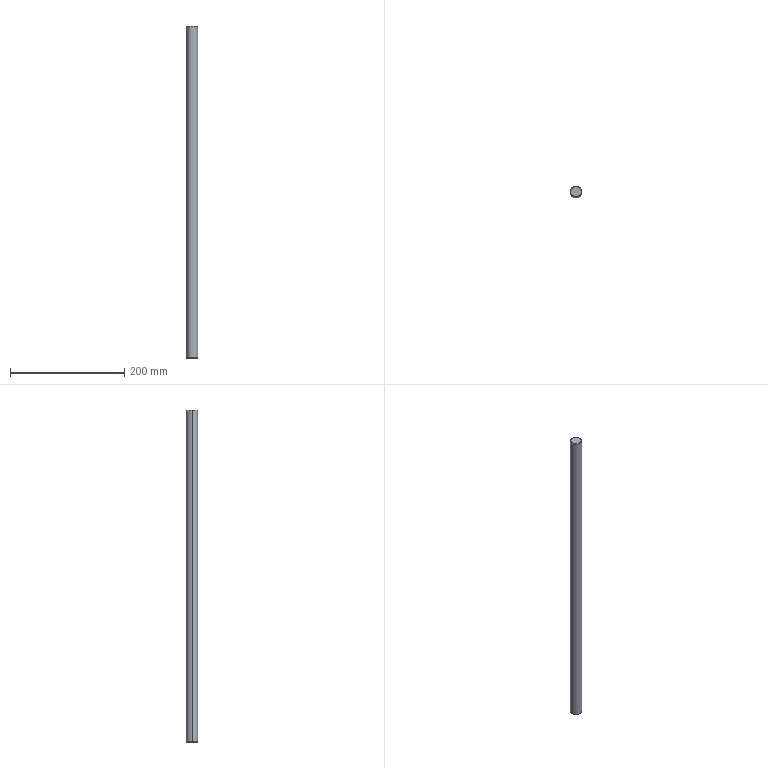Part | STEP file | 20309 | 1 solid | 8 faces | box 20 x 20 x 580 mm | volume 182152 mm3 | cone 4 | plane 2 | cylinder 2 | commonest cylinder face diameters 20 x2
STEP:
#1=CARTESIAN_POINT('',(9.,0.,580.));
#2=VERTEX_POINT('',#1);
#3=CARTESIAN_POINT('',(-9.,0.000000111,580.));
#4=VERTEX_POINT('',#3);
#5=CARTESIAN_POINT('',(0.,0.,580.));
#6=DIRECTION('',(0.,0.,1.));
#7=AXIS2_PLACEMENT_3D('',#5,#6,$);
#8=CIRCLE('',#7,9.);
#9=EDGE_CURVE('',#2,#4,#8,.T.);
#10=ORIENTED_EDGE('',*,*,#9,.T.);
#11=CARTESIAN_POINT('',(0.,0.,580.));
#12=DIRECTION('',(0.,0.,1.));
#13=AXIS2_PLACEMENT_3D('',#11,#12,$);
#14=CIRCLE('',#13,9.);
#15=EDGE_CURVE('',#4,#2,#14,.T.);
#16=ORIENTED_EDGE('',*,*,#15,.T.);
#17=EDGE_LOOP('',(#10,#16));
#18=FACE_OUTER_BOUND('',#17,.T.);
#19=CARTESIAN_POINT('',(0.,0.,580.));
#20=DIRECTION('',(0.,0.,1.));
#21=DIRECTION('',(1.,0.,0.));
#22=AXIS2_PLACEMENT_3D('',#19,#20,#21);
#23=PLANE('',#22);
#24=ADVANCED_FACE('',(#18),#23,.T.);
#25=CARTESIAN_POINT('',(10.,0.,579.));
#26=VERTEX_POINT('',#25);
#27=CARTESIAN_POINT('',(9.5,0.,579.5));
#28=DIRECTION('',(0.7071,0.,-0.7071));
#29=VECTOR('',#28,1.);
#30=LINE('',#27,#29);
#31=EDGE_CURVE('',#2,#26,#30,.T.);
#32=ORIENTED_EDGE('',*,*,#31,.T.);
#33=CARTESIAN_POINT('',(-10.,0.,579.));
#34=VERTEX_POINT('',#33);
#35=CARTESIAN_POINT('',(0.,0.,579.));
#36=DIRECTION('',(0.,0.,1.));
#37=AXIS2_PLACEMENT_3D('',#35,#36,$);
#38=CIRCLE('',#37,10.);
#39=EDGE_CURVE('',#26,#34,#38,.T.);
#40=ORIENTED_EDGE('',*,*,#39,.T.);
#41=CARTESIAN_POINT('',(-9.5,0.,579.5));
#42=DIRECTION('',(-0.7071,0.,-0.7071));
#43=VECTOR('',#42,1.);
#44=LINE('',#41,#43);
#45=EDGE_CURVE('',#4,#34,#44,.T.);
#46=ORIENTED_EDGE('',*,*,#45,.F.);
#47=ORIENTED_EDGE('',*,*,#9,.F.);
#48=EDGE_LOOP('',(#32,#40,#46,#47));
#49=FACE_OUTER_BOUND('',#48,.T.);
#50=CARTESIAN_POINT('',(0.,0.,589.));
#51=DIRECTION('',(0.,0.,-1.));
#52=DIRECTION('',(1.,0.,0.));
#53=AXIS2_PLACEMENT_3D('',#50,#51,#52);
#54=CONICAL_SURFACE('',#53,0.,0.7854);
#55=ADVANCED_FACE('',(#49),#54,.T.);
#56=ORIENTED_EDGE('',*,*,#45,.T.);
#57=CARTESIAN_POINT('',(0.,0.,579.));
#58=DIRECTION('',(0.,0.,1.));
#59=AXIS2_PLACEMENT_3D('',#57,#58,$);
#60=CIRCLE('',#59,10.);
#61=EDGE_CURVE('',#34,#26,#60,.T.);
#62=ORIENTED_EDGE('',*,*,#61,.T.);
#63=ORIENTED_EDGE('',*,*,#31,.F.);
#64=ORIENTED_EDGE('',*,*,#15,.F.);
#65=EDGE_LOOP('',(#56,#62,#63,#64));
#66=FACE_OUTER_BOUND('',#65,.T.);
#67=CARTESIAN_POINT('',(0.,0.,589.));
#68=DIRECTION('',(0.,0.,-1.));
#69=DIRECTION('',(-0.9881,0.1539,0.));
#70=AXIS2_PLACEMENT_3D('',#67,#68,#69);
#71=CONICAL_SURFACE('',#70,0.,0.7854);
#72=ADVANCED_FACE('',(#66),#71,.T.);
#73=CARTESIAN_POINT('',(-9.,0.000000111,0.));
#74=VERTEX_POINT('',#73);
#75=CARTESIAN_POINT('',(9.,0.,0.));
#76=VERTEX_POINT('',#75);
#77=CARTESIAN_POINT('',(0.,0.,0.));
#78=DIRECTION('',(0.,0.,1.));
#79=AXIS2_PLACEMENT_3D('',#77,#78,$);
#80=CIRCLE('',#79,9.);
#81=EDGE_CURVE('',#74,#76,#80,.T.);
#82=ORIENTED_EDGE('',*,*,#81,.F.);
#83=CARTESIAN_POINT('',(0.,0.,0.));
#84=DIRECTION('',(0.,0.,1.));
#85=AXIS2_PLACEMENT_3D('',#83,#84,$);
#86=CIRCLE('',#85,9.);
#87=EDGE_CURVE('',#76,#74,#86,.T.);
#88=ORIENTED_EDGE('',*,*,#87,.F.);
#89=EDGE_LOOP('',(#82,#88));
#90=FACE_OUTER_BOUND('',#89,.T.);
#91=CARTESIAN_POINT('',(0.,0.,0.));
#92=DIRECTION('',(0.,0.,1.));
#93=DIRECTION('',(1.,0.,0.));
#94=AXIS2_PLACEMENT_3D('',#91,#92,#93);
#95=PLANE('',#94);
#96=ADVANCED_FACE('',(#90),#95,.F.);
#97=CARTESIAN_POINT('',(-10.,0.,1.));
#98=VERTEX_POINT('',#97);
#99=CARTESIAN_POINT('',(-10.,0.,290.));
#100=DIRECTION('',(0.,0.,1.));
#101=VECTOR('',#100,1.);
#102=LINE('',#99,#101);
#103=EDGE_CURVE('',#98,#34,#102,.T.);
#104=ORIENTED_EDGE('',*,*,#103,.T.);
#105=ORIENTED_EDGE('',*,*,#39,.F.);
#106=CARTESIAN_POINT('',(10.,0.,1.));
#107=VERTEX_POINT('',#106);
#108=CARTESIAN_POINT('',(10.,0.,290.));
#109=DIRECTION('',(0.,0.,1.));
#110=VECTOR('',#109,1.);
#111=LINE('',#108,#110);
#112=EDGE_CURVE('',#107,#26,#111,.T.);
#113=ORIENTED_EDGE('',*,*,#112,.F.);
#114=CARTESIAN_POINT('',(0.,0.,1.));
#115=DIRECTION('',(0.,0.,1.));
#116=AXIS2_PLACEMENT_3D('',#114,#115,$);
#117=CIRCLE('',#116,10.);
#118=EDGE_CURVE('',#107,#98,#117,.T.);
#119=ORIENTED_EDGE('',*,*,#118,.T.);
#120=EDGE_LOOP('',(#104,#105,#113,#119));
#121=FACE_OUTER_BOUND('',#120,.T.);
#122=CARTESIAN_POINT('',(0.,0.,290.));
#123=DIRECTION('',(0.,0.,1.));
#124=DIRECTION('',(1.,0.,0.));
#125=AXIS2_PLACEMENT_3D('',#122,#123,#124);
#126=CYLINDRICAL_SURFACE('',#125,10.);
#127=ADVANCED_FACE('',(#121),#126,.T.);
#128=ORIENTED_EDGE('',*,*,#112,.T.);
#129=ORIENTED_EDGE('',*,*,#61,.F.);
#130=ORIENTED_EDGE('',*,*,#103,.F.);
#131=CARTESIAN_POINT('',(0.,0.,1.));
#132=DIRECTION('',(0.,0.,1.));
#133=AXIS2_PLACEMENT_3D('',#131,#132,$);
#134=CIRCLE('',#133,10.);
#135=EDGE_CURVE('',#98,#107,#134,.T.);
#136=ORIENTED_EDGE('',*,*,#135,.T.);
#137=EDGE_LOOP('',(#128,#129,#130,#136));
#138=FACE_OUTER_BOUND('',#137,.T.);
#139=ADVANCED_FACE('',(#138),#126,.T.);
#140=CARTESIAN_POINT('',(9.5,0.,0.5));
#141=DIRECTION('',(0.7071,0.,0.7071));
#142=VECTOR('',#141,1.);
#143=LINE('',#140,#142);
#144=EDGE_CURVE('',#107,#76,#143,.F.);
#145=ORIENTED_EDGE('',*,*,#144,.T.);
#146=ORIENTED_EDGE('',*,*,#87,.T.);
#147=CARTESIAN_POINT('',(-9.5,0.000000117,0.5));
#148=DIRECTION('',(-0.7071,0.000000009,0.7071));
#149=VECTOR('',#148,1.);
#150=LINE('',#147,#149);
#151=EDGE_CURVE('',#98,#74,#150,.F.);
#152=ORIENTED_EDGE('',*,*,#151,.F.);
#153=ORIENTED_EDGE('',*,*,#118,.F.);
#154=EDGE_LOOP('',(#145,#146,#152,#153));
#155=FACE_OUTER_BOUND('',#154,.T.);
#156=CARTESIAN_POINT('',(0.,0.,-9.));
#157=DIRECTION('',(0.,0.,1.));
#158=DIRECTION('',(1.,0.,0.));
#159=AXIS2_PLACEMENT_3D('',#156,#157,#158);
#160=CONICAL_SURFACE('',#159,0.,0.7854);
#161=ADVANCED_FACE('',(#155),#160,.T.);
#162=ORIENTED_EDGE('',*,*,#151,.T.);
#163=ORIENTED_EDGE('',*,*,#81,.T.);
#164=ORIENTED_EDGE('',*,*,#144,.F.);
#165=ORIENTED_EDGE('',*,*,#135,.F.);
#166=EDGE_LOOP('',(#162,#163,#164,#165));
#167=FACE_OUTER_BOUND('',#166,.T.);
#168=CARTESIAN_POINT('',(0.,0.,-9.));
#169=DIRECTION('',(0.,0.,1.));
#170=DIRECTION('',(-0.9881,0.1539,0.));
#171=AXIS2_PLACEMENT_3D('',#168,#169,#170);
#172=CONICAL_SURFACE('',#171,0.,0.7854);
#173=ADVANCED_FACE('',(#167),#172,.T.);
#174=CLOSED_SHELL('',(#24,#55,#72,#96,#127,#139,#161,#173));
#175=MANIFOLD_SOLID_BREP('',#174);
#176=(LENGTH_UNIT()NAMED_UNIT(*)SI_UNIT(.MILLI.,.METRE.));
#177=UNCERTAINTY_MEASURE_WITH_UNIT(LENGTH_MEASURE(0.005),#176,'','');
#178=(NAMED_UNIT(*)PLANE_ANGLE_UNIT()SI_UNIT($,.RADIAN.));
#179=(NAMED_UNIT(*)SI_UNIT($,.STERADIAN.)SOLID_ANGLE_UNIT());
#180=(GEOMETRIC_REPRESENTATION_CONTEXT(3)GLOBAL_UNCERTAINTY_ASSIGNED_CONTEXT((#177))GLOBAL_UNIT_ASSIGNED_CONTEXT((#176,#178,#179))REPRESENTATION_CONTEXT('',''));
#181=ADVANCED_BREP_SHAPE_REPRESENTATION('',(#175),#180);